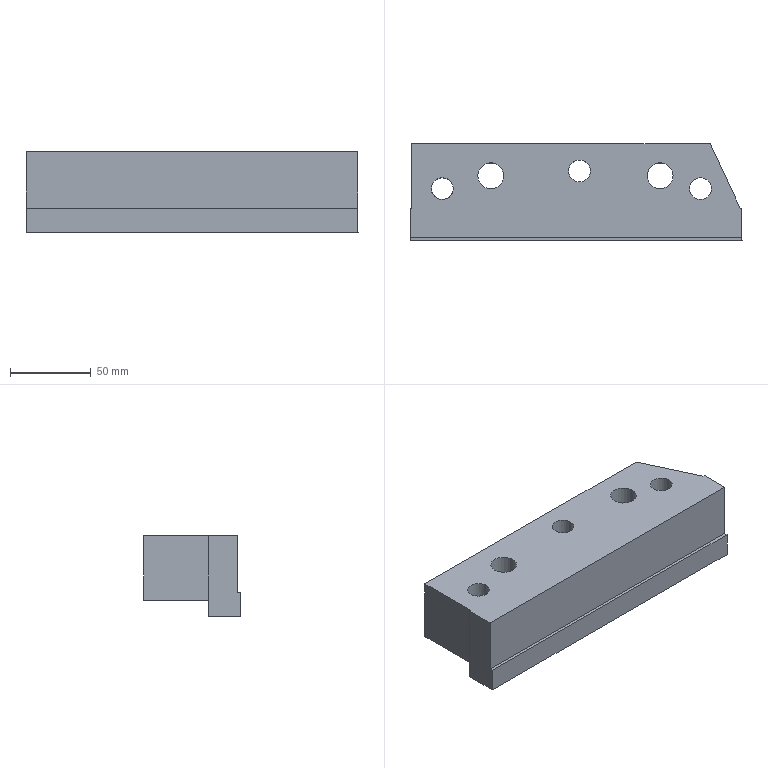Part | NX | features solid 2 | 1 solid | 23 faces | box 205.676 x 60.004 x 50 mm | volume 461052 mm3 | plane 12 | cylinder 8 | spline 3 | commonest cylinder face diameters 13.5 x3 19.5 x3 16 x2
STEP:
#1=CARTESIAN_POINT('',(205.675,-58.001,43.));
#2=VERTEX_POINT('',#1);
#3=CARTESIAN_POINT('',(205.675,-58.001,8.));
#4=VERTEX_POINT('',#3);
#5=CARTESIAN_POINT('',(205.675,-58.001,25.5));
#6=DIRECTION('',(0.,0.,-1.));
#7=VECTOR('',#6,1000.);
#8=LINE('',#5,#7);
#9=EDGE_CURVE('',#2,#4,#8,.T.);
#10=ORIENTED_EDGE('',*,*,#9,.F.);
#11=CARTESIAN_POINT('',(0.,-58.,43.));
#12=VERTEX_POINT('',#11);
#13=CARTESIAN_POINT('',(205.675,-58.001,43.));
#14=CARTESIAN_POINT('',(137.117,-58.009,43.));
#15=CARTESIAN_POINT('',(68.559,-58.,43.));
#16=CARTESIAN_POINT('',(0.,-58.,43.));
#17=B_SPLINE_CURVE_WITH_KNOTS('',3,(#13,#14,#15,#16),.UNSPECIFIED.,.F.,.F.,(4,4),(0.7842,1.),.UNSPECIFIED.);
#18=EDGE_CURVE('',#2,#12,#17,.T.);
#19=ORIENTED_EDGE('',*,*,#18,.T.);
#20=CARTESIAN_POINT('',(0.,-58.,8.));
#21=VERTEX_POINT('',#20);
#22=CARTESIAN_POINT('',(0.,-58.,25.5));
#23=DIRECTION('',(0.,0.,-1.));
#24=VECTOR('',#23,1000.);
#25=LINE('',#22,#24);
#26=EDGE_CURVE('',#12,#21,#25,.T.);
#27=ORIENTED_EDGE('',*,*,#26,.T.);
#28=CARTESIAN_POINT('',(205.675,-58.001,8.));
#29=CARTESIAN_POINT('',(137.117,-58.009,8.));
#30=CARTESIAN_POINT('',(68.559,-58.,8.));
#31=CARTESIAN_POINT('',(0.,-58.,8.));
#32=B_SPLINE_CURVE_WITH_KNOTS('',3,(#28,#29,#30,#31),.UNSPECIFIED.,.F.,.F.,(4,4),(0.7842,1.),.UNSPECIFIED.);
#33=EDGE_CURVE('',#4,#21,#32,.T.);
#34=ORIENTED_EDGE('',*,*,#33,.F.);
#35=EDGE_LOOP('',(#10,#19,#27,#34));
#36=FACE_BOUND('',#35,.T.);
#37=CARTESIAN_POINT('',(205.675,-58.001,43.));
#38=CARTESIAN_POINT('',(205.675,-58.001,8.));
#39=CARTESIAN_POINT('',(137.117,-58.009,43.));
#40=CARTESIAN_POINT('',(137.117,-58.009,8.));
#41=CARTESIAN_POINT('',(68.559,-58.,43.));
#42=CARTESIAN_POINT('',(68.559,-58.,8.));
#43=CARTESIAN_POINT('',(0.,-58.,43.));
#44=CARTESIAN_POINT('',(0.,-58.,8.));
#45=B_SPLINE_SURFACE_WITH_KNOTS('',3,1,((#37,#38),(#39,#40),(#41,#42),(#43,#44)),.SURF_OF_LINEAR_EXTRUSION.,.F.,.F.,.F.,(4,4),(2,2),(0.7842,1.),(0.,1.),.PIECEWISE_BEZIER_KNOTS.);
#46=ADVANCED_FACE('',(#36),#45,.T.);
#47=CARTESIAN_POINT('',(58.,-20.,43.));
#48=VERTEX_POINT('',#47);
#49=CARTESIAN_POINT('',(50.,-20.,43.));
#50=DIRECTION('',(0.,0.,1.));
#51=DIRECTION('',(1.,0.,0.));
#52=AXIS2_PLACEMENT_3D('',#49,#50,#51);
#53=CIRCLE('',#52,8.);
#54=EDGE_CURVE('',#48,#48,#53,.T.);
#55=ORIENTED_EDGE('',*,*,#54,.F.);
#56=EDGE_LOOP('',(#55));
#57=FACE_BOUND('',#56,.T.);
#58=CARTESIAN_POINT('',(147.,-20.,43.));
#59=VERTEX_POINT('',#58);
#60=CARTESIAN_POINT('',(155.,-20.,43.));
#61=DIRECTION('',(0.,0.,-1.));
#62=DIRECTION('',(-1.,0.,0.));
#63=AXIS2_PLACEMENT_3D('',#60,#61,#62);
#64=CIRCLE('',#63,8.);
#65=EDGE_CURVE('',#59,#59,#64,.T.);
#66=ORIENTED_EDGE('',*,*,#65,.T.);
#67=EDGE_LOOP('',(#66));
#68=FACE_BOUND('',#67,.T.);
#69=CARTESIAN_POINT('',(26.75,-28.,43.));
#70=VERTEX_POINT('',#69);
#71=CARTESIAN_POINT('',(20.,-28.,43.));
#72=DIRECTION('',(0.,0.,1.));
#73=DIRECTION('',(1.,0.,0.));
#74=AXIS2_PLACEMENT_3D('',#71,#72,#73);
#75=CIRCLE('',#74,6.75);
#76=EDGE_CURVE('',#70,#70,#75,.T.);
#77=ORIENTED_EDGE('',*,*,#76,.F.);
#78=EDGE_LOOP('',(#77));
#79=FACE_BOUND('',#78,.T.);
#80=CARTESIAN_POINT('',(98.25,-17.,43.));
#81=VERTEX_POINT('',#80);
#82=CARTESIAN_POINT('',(105.,-17.,43.));
#83=DIRECTION('',(0.,0.,-1.));
#84=DIRECTION('',(-1.,0.,0.));
#85=AXIS2_PLACEMENT_3D('',#82,#83,#84);
#86=CIRCLE('',#85,6.75);
#87=EDGE_CURVE('',#81,#81,#86,.T.);
#88=ORIENTED_EDGE('',*,*,#87,.T.);
#89=EDGE_LOOP('',(#88));
#90=FACE_BOUND('',#89,.T.);
#91=CARTESIAN_POINT('',(173.25,-28.,43.));
#92=VERTEX_POINT('',#91);
#93=CARTESIAN_POINT('',(180.,-28.,43.));
#94=DIRECTION('',(0.,0.,-1.));
#95=DIRECTION('',(-1.,0.,0.));
#96=AXIS2_PLACEMENT_3D('',#93,#94,#95);
#97=CIRCLE('',#96,6.75);
#98=EDGE_CURVE('',#92,#92,#97,.T.);
#99=ORIENTED_EDGE('',*,*,#98,.T.);
#100=EDGE_LOOP('',(#99));
#101=FACE_BOUND('',#100,.T.);
#102=CARTESIAN_POINT('',(1.,-40.,43.));
#103=VERTEX_POINT('',#102);
#104=CARTESIAN_POINT('',(1.,0.,43.));
#105=VERTEX_POINT('',#104);
#106=CARTESIAN_POINT('',(1.,-1.,43.));
#107=DIRECTION('',(0.,1.,0.));
#108=VECTOR('',#107,1000.);
#109=LINE('',#106,#108);
#110=EDGE_CURVE('',#103,#105,#109,.T.);
#111=ORIENTED_EDGE('',*,*,#110,.F.);
#112=CARTESIAN_POINT('',(0.,-40.,43.));
#113=VERTEX_POINT('',#112);
#114=CARTESIAN_POINT('',(0.,-40.,43.));
#115=CARTESIAN_POINT('',(0.3333,-40.,43.));
#116=CARTESIAN_POINT('',(0.6667,-40.,43.));
#117=CARTESIAN_POINT('',(1.,-40.,43.));
#118=B_SPLINE_CURVE_WITH_KNOTS('',3,(#114,#115,#116,#117),.UNSPECIFIED.,.F.,.F.,(4,4),(0.,0.001),.UNSPECIFIED.);
#119=EDGE_CURVE('',#103,#113,#118,.F.);
#120=ORIENTED_EDGE('',*,*,#119,.T.);
#121=CARTESIAN_POINT('',(0.,0.,43.));
#122=DIRECTION('',(0.,-1.,0.));
#123=VECTOR('',#122,1000.);
#124=LINE('',#121,#123);
#125=EDGE_CURVE('',#113,#12,#124,.T.);
#126=ORIENTED_EDGE('',*,*,#125,.T.);
#127=ORIENTED_EDGE('',*,*,#18,.F.);
#128=CARTESIAN_POINT('',(205.675,-40.001,43.));
#129=VERTEX_POINT('',#128);
#130=CARTESIAN_POINT('',(205.668,84.753,43.));
#131=DIRECTION('',(0.00005304,-1.,0.));
#132=VECTOR('',#131,1000.);
#133=LINE('',#130,#132);
#134=EDGE_CURVE('',#129,#2,#133,.T.);
#135=ORIENTED_EDGE('',*,*,#134,.F.);
#136=CARTESIAN_POINT('',(204.571,-40.001,43.));
#137=VERTEX_POINT('',#136);
#138=CARTESIAN_POINT('',(205.675,-40.001,43.));
#139=CARTESIAN_POINT('',(205.307,-40.001,43.));
#140=CARTESIAN_POINT('',(204.939,-40.001,43.));
#141=CARTESIAN_POINT('',(204.571,-40.001,43.));
#142=B_SPLINE_CURVE_WITH_KNOTS('',3,(#138,#139,#140,#141),.UNSPECIFIED.,.F.,.F.,(4,4),(0.,0.001103),.UNSPECIFIED.);
#143=EDGE_CURVE('',#129,#137,#142,.T.);
#144=ORIENTED_EDGE('',*,*,#143,.T.);
#145=CARTESIAN_POINT('',(185.918,0.,43.));
#146=VERTEX_POINT('',#145);
#147=CARTESIAN_POINT('',(186.538,-1.329,43.));
#148=DIRECTION('',(0.4226,-0.9063,0.));
#149=VECTOR('',#148,1000.);
#150=LINE('',#147,#149);
#151=EDGE_CURVE('',#137,#146,#150,.F.);
#152=ORIENTED_EDGE('',*,*,#151,.T.);
#153=CARTESIAN_POINT('',(0.,0.,43.));
#154=DIRECTION('',(1.,0.,0.));
#155=VECTOR('',#154,1000.);
#156=LINE('',#153,#155);
#157=EDGE_CURVE('',#105,#146,#156,.T.);
#158=ORIENTED_EDGE('',*,*,#157,.F.);
#159=EDGE_LOOP('',(#111,#120,#126,#127,#135,#144,#152,#158));
#160=FACE_BOUND('',#159,.T.);
#161=CARTESIAN_POINT('',(396.872,84.764,43.));
#162=DIRECTION('',(0.,0.,-1.));
#163=DIRECTION('',(1.,0.,0.));
#164=AXIS2_PLACEMENT_3D('',#161,#162,#163);
#165=PLANE('',#164);
#166=ADVANCED_FACE('',(#57,#68,#79,#90,#101,#160),#165,.F.);
#167=CARTESIAN_POINT('',(205.675,-40.001,-7.));
#168=VERTEX_POINT('',#167);
#169=CARTESIAN_POINT('',(70.,-40.002,-7.));
#170=VERTEX_POINT('',#169);
#171=CARTESIAN_POINT('',(222.421,-40.,-7.));
#172=CARTESIAN_POINT('',(215.62,-40.001,-7.));
#173=CARTESIAN_POINT('',(208.82,-40.001,-7.));
#174=CARTESIAN_POINT('',(202.019,-40.001,-7.));
#175=CARTESIAN_POINT('',(201.346,-40.001,-7.));
#176=CARTESIAN_POINT('',(200.672,-40.001,-7.));
#177=CARTESIAN_POINT('',(199.999,-40.001,-7.));
#178=CARTESIAN_POINT('',(185.832,-40.002,-7.));
#179=CARTESIAN_POINT('',(171.666,-40.003,-7.));
#180=CARTESIAN_POINT('',(143.333,-40.004,-7.));
#181=CARTESIAN_POINT('',(129.167,-40.003,-7.));
#182=CARTESIAN_POINT('',(95.834,-40.003,-7.));
#183=CARTESIAN_POINT('',(76.667,-40.002,-7.));
#184=CARTESIAN_POINT('',(38.334,-40.,-7.));
#185=CARTESIAN_POINT('',(19.167,-40.,-7.));
#186=CARTESIAN_POINT('',(0.000401,-40.,-7.));
#187=CARTESIAN_POINT('',(-0.6663,-40.,-7.));
#188=CARTESIAN_POINT('',(-1.333,-40.,-7.));
#189=CARTESIAN_POINT('',(-2.,-40.,-7.));
#190=B_SPLINE_CURVE_WITH_KNOTS('',3,(#171,#172,#173,#174,#175,#176,#177,#178,#179,#180,#181,#182,#183,#184,#185,#186,#187,#188,#189),.UNSPECIFIED.,.F.,.F.,(4,3,3,2,2,2,3,4),(-0.1121,-0.0101,0.,0.2125,0.425,0.7125,1.,1.01),.UNSPECIFIED.);
#191=EDGE_CURVE('',#168,#170,#190,.T.);
#192=ORIENTED_EDGE('',*,*,#191,.F.);
#193=CARTESIAN_POINT('',(205.676,-60.001,-7.));
#194=VERTEX_POINT('',#193);
#195=CARTESIAN_POINT('',(205.668,84.753,-7.));
#196=DIRECTION('',(0.00005304,-1.,0.));
#197=VECTOR('',#196,1000.);
#198=LINE('',#195,#197);
#199=EDGE_CURVE('',#168,#194,#198,.T.);
#200=ORIENTED_EDGE('',*,*,#199,.T.);
#201=CARTESIAN_POINT('',(70.,-60.002,-7.));
#202=VERTEX_POINT('',#201);
#203=CARTESIAN_POINT('',(704.143,549.489,-7.));
#204=CARTESIAN_POINT('',(700.294,502.993,-7.));
#205=CARTESIAN_POINT('',(696.445,456.496,-7.));
#206=CARTESIAN_POINT('',(692.595,410.,-7.));
#207=CARTESIAN_POINT('',(692.458,408.343,-7.));
#208=CARTESIAN_POINT('',(692.134,405.032,-7.));
#209=CARTESIAN_POINT('',(691.827,400.886,-7.));
#210=CARTESIAN_POINT('',(691.464,397.578,-7.));
#211=CARTESIAN_POINT('',(691.402,395.086,-7.));
#212=CARTESIAN_POINT('',(690.964,392.595,-7.));
#213=CARTESIAN_POINT('',(689.408,390.517,-7.));
#214=CARTESIAN_POINT('',(686.986,389.671,-7.));
#215=CARTESIAN_POINT('',(684.487,389.581,-7.));
#216=CARTESIAN_POINT('',(681.996,389.453,-7.));
#217=CARTESIAN_POINT('',(678.704,388.96,-7.));
#218=CARTESIAN_POINT('',(674.57,388.503,-7.));
#219=CARTESIAN_POINT('',(669.673,387.535,-7.));
#220=CARTESIAN_POINT('',(664.783,386.537,-7.));
#221=CARTESIAN_POINT('',(659.995,385.127,-7.));
#222=CARTESIAN_POINT('',(655.202,383.733,-7.));
#223=CARTESIAN_POINT('',(650.55,381.923,-7.));
#224=CARTESIAN_POINT('',(646.672,380.42,-7.));
#225=CARTESIAN_POINT('',(643.662,379.005,-7.));
#226=CARTESIAN_POINT('',(641.411,377.928,-7.));
#227=CARTESIAN_POINT('',(639.156,376.862,-7.));
#228=CARTESIAN_POINT('',(636.191,375.356,-7.));
#229=CARTESIAN_POINT('',(632.576,373.295,-7.));
#230=CARTESIAN_POINT('',(629.081,371.043,-7.));
#231=CARTESIAN_POINT('',(626.283,369.244,-7.));
#232=CARTESIAN_POINT('',(624.228,367.832,-7.));
#233=CARTESIAN_POINT('',(622.21,366.363,-7.));
#234=CARTESIAN_POINT('',(619.546,364.372,-7.));
#235=CARTESIAN_POINT('',(616.368,361.691,-7.));
#236=CARTESIAN_POINT('',(612.546,358.478,-7.));
#237=CARTESIAN_POINT('',(609.042,354.922,-7.));
#238=CARTESIAN_POINT('',(606.061,352.022,-7.));
#239=CARTESIAN_POINT('',(603.887,349.505,-7.));
#240=CARTESIAN_POINT('',(602.262,347.611,-7.));
#241=CARTESIAN_POINT('',(600.634,345.722,-7.));
#242=CARTESIAN_POINT('',(598.542,343.136,-7.));
#243=CARTESIAN_POINT('',(594.998,338.518,-7.));
#244=CARTESIAN_POINT('',(589.869,331.973,-7.));
#245=CARTESIAN_POINT('',(583.732,324.105,-7.));
#246=CARTESIAN_POINT('',(578.643,317.53,-7.));
#247=CARTESIAN_POINT('',(574.554,312.279,-7.));
#248=CARTESIAN_POINT('',(570.923,306.701,-7.));
#249=CARTESIAN_POINT('',(564.822,296.785,-7.));
#250=CARTESIAN_POINT('',(557.245,281.952,-7.));
#251=CARTESIAN_POINT('',(551.45,266.325,-7.));
#252=CARTESIAN_POINT('',(548.558,255.043,-7.));
#253=CARTESIAN_POINT('',(547.23,248.523,-7.));
#254=CARTESIAN_POINT('',(546.404,243.602,-7.));
#255=CARTESIAN_POINT('',(545.685,238.665,-7.));
#256=CARTESIAN_POINT('',(544.956,233.729,-7.));
#257=CARTESIAN_POINT('',(544.163,228.804,-7.));
#258=CARTESIAN_POINT('',(543.03,222.238,-7.));
#259=CARTESIAN_POINT('',(540.604,216.007,-7.));
#260=CARTESIAN_POINT('',(537.562,210.084,-7.));
#261=CARTESIAN_POINT('',(534.784,205.926,-7.));
#262=CARTESIAN_POINT('',(532.049,202.788,-7.));
#263=CARTESIAN_POINT('',(529.701,200.432,-7.));
#264=CARTESIAN_POINT('',(527.298,198.128,-7.));
#265=CARTESIAN_POINT('',(524.699,196.054,-7.));
#266=CARTESIAN_POINT('',(521.947,194.18,-7.));
#267=CARTESIAN_POINT('',(519.13,192.405,-7.));
#268=CARTESIAN_POINT('',(515.609,190.197,-7.));
#269=CARTESIAN_POINT('',(509.995,186.628,-7.));
#270=CARTESIAN_POINT('',(505.193,183.605,-7.));
#271=CARTESIAN_POINT('',(488.347,172.979,-7.));
#272=CARTESIAN_POINT('',(470.923,162.051,-7.));
#273=CARTESIAN_POINT('',(452.433,150.371,-7.));
#274=CARTESIAN_POINT('',(445.662,146.198,-7.));
#275=CARTESIAN_POINT('',(440.606,143.035,-7.));
#276=CARTESIAN_POINT('',(435.698,139.633,-7.));
#277=CARTESIAN_POINT('',(429.565,134.565,-7.));
#278=CARTESIAN_POINT('',(422.879,127.153,-7.));
#279=CARTESIAN_POINT('',(416.014,117.403,-7.));
#280=CARTESIAN_POINT('',(409.871,107.153,-7.));
#281=CARTESIAN_POINT('',(404.995,98.493,-7.));
#282=CARTESIAN_POINT('',(400.982,91.628,-7.));
#283=CARTESIAN_POINT('',(394.857,81.39,-7.));
#284=CARTESIAN_POINT('',(385.627,66.06,-7.));
#285=CARTESIAN_POINT('',(373.359,45.597,-7.));
#286=CARTESIAN_POINT('',(361.076,25.143,-7.));
#287=CARTESIAN_POINT('',(351.863,9.803,-7.));
#288=CARTESIAN_POINT('',(346.247,0.4191,-7.));
#289=CARTESIAN_POINT('',(344.171,-2.972,-7.));
#290=CARTESIAN_POINT('',(342.561,-5.482,-7.));
#291=CARTESIAN_POINT('',(340.921,-7.974,-7.));
#292=CARTESIAN_POINT('',(338.671,-11.253,-7.));
#293=CARTESIAN_POINT('',(335.579,-15.149,-7.));
#294=CARTESIAN_POINT('',(331.771,-19.742,-7.));
#295=CARTESIAN_POINT('',(327.68,-24.086,-7.));
#296=CARTESIAN_POINT('',(323.394,-28.235,-7.));
#297=CARTESIAN_POINT('',(318.933,-32.197,-7.));
#298=CARTESIAN_POINT('',(315.035,-35.286,-7.));
#299=CARTESIAN_POINT('',(311.798,-37.595,-7.));
#300=CARTESIAN_POINT('',(308.565,-39.911,-7.));
#301=CARTESIAN_POINT('',(304.4,-42.633,-7.));
#302=CARTESIAN_POINT('',(299.148,-45.464,-7.));
#303=CARTESIAN_POINT('',(293.89,-48.284,-7.));
#304=CARTESIAN_POINT('',(289.325,-50.258,-7.));
#305=CARTESIAN_POINT('',(285.634,-51.738,-7.));
#306=CARTESIAN_POINT('',(282.879,-52.885,-7.));
#307=CARTESIAN_POINT('',(280.041,-53.8,-7.));
#308=CARTESIAN_POINT('',(277.185,-54.663,-7.));
#309=CARTESIAN_POINT('',(274.33,-55.522,-7.));
#310=CARTESIAN_POINT('',(270.488,-56.55,-7.));
#311=CARTESIAN_POINT('',(265.653,-57.72,-7.));
#312=CARTESIAN_POINT('',(260.737,-58.464,-7.));
#313=CARTESIAN_POINT('',(256.804,-59.062,-7.));
#314=CARTESIAN_POINT('',(254.337,-59.354,-7.));
#315=CARTESIAN_POINT('',(252.356,-59.521,-7.));
#316=CARTESIAN_POINT('',(250.373,-59.675,-7.));
#317=CARTESIAN_POINT('',(247.891,-59.803,-7.));
#318=CARTESIAN_POINT('',(244.911,-59.906,-7.));
#319=CARTESIAN_POINT('',(240.936,-60.021,-7.));
#320=CARTESIAN_POINT('',(235.965,-60.032,-7.));
#321=CARTESIAN_POINT('',(231.03,-59.997,-7.));
#322=CARTESIAN_POINT('',(190.708,-60.004,-7.));
#323=CARTESIAN_POINT('',(114.042,-60.004,-7.));
#324=CARTESIAN_POINT('',(38.333,-60.,-7.));
#325=CARTESIAN_POINT('',(0.,-60.,-7.));
#326=CARTESIAN_POINT('',(-46.656,-60.,-7.));
#327=CARTESIAN_POINT('',(-93.311,-60.,-7.));
#328=CARTESIAN_POINT('',(-139.967,-60.,-7.));
#329=B_SPLINE_CURVE_WITH_KNOTS('',3,(#203,#204,#205,#206,#207,#208,#209,#210,#211,#212,#213,#214,#215,#216,#217,#218,#219,#220,#221,#222,#223,#224,#225,#226,#227,#228,#229,#230,#231,#232,#233,#234,#235,#236,#237,#238,#239,#240,#241,#242,#243,#244,#245,#246,#247,#248,#249,#250,#251,#252,#253,#254,#255,#256,#257,#258,#259,#260,#261,#262,#263,#264,#265,#266,#267,#268,#269,#270,#271,#272,#273,#274,#275,#276,#277,#278,#279,#280,#281,#282,#283,#284,#285,#286,#287,#288,#289,#290,#291,#292,#293,#294,#295,#296,#297,#298,#299,#300,#301,#302,#303,#304,#305,#306,#307,#308,#309,#310,#311,#312,#313,#314,#315,#316,#317,#318,#319,#320,#321,#322,#323,#324,#325,#326,#327,#328),.UNSPECIFIED.,.F.,.F.,(4,3,1,1,1,1,1,1,1,1,1,1,1,1,1,1,1,1,1,1,1,1,1,1,1,1,1,1,1,1,1,1,1,1,1,1,1,1,1,1,1,1,1,1,1,1,1,1,1,1,1,1,1,1,1,1,1,1,1,1,1,1,1,1,1,1,1,1,1,1,1,1,1,1,1,1,1,1,1,1,1,1,1,1,1,1,1,1,1,1,1,1,1,1,1,1,1,1,1,1,1,1,1,1,1,1,1,1,1,1,1,1,1,1,1,1,1,1,3,4),(-0.15,0.,0.005347,0.01069,0.01337,0.01604,0.01871,0.02139,0.02406,0.02673,0.02941,0.03208,0.03743,0.04278,0.04812,0.05347,0.05882,0.06416,0.06951,0.07218,0.07486,0.07753,0.0802,0.08555,0.0909,0.09357,0.09624,0.09892,0.1016,0.1069,0.1123,0.1176,0.123,0.1257,0.1283,0.131,0.1337,0.139,0.1497,0.1604,0.1711,0.1764,0.1818,0.1925,0.2139,0.2353,0.246,0.2513,0.2567,0.262,0.2673,0.2727,0.278,0.2887,0.2941,0.2994,0.3048,0.3074,0.3101,0.3155,0.3181,0.3208,0.3262,0.3315,0.3422,0.3444,0.3955,0.4083,0.4147,0.4211,0.4275,0.4339,0.4467,0.4595,0.4722,0.485,0.4914,0.4978,0.5234,0.549,0.5745,0.6001,0.6065,0.6097,0.6129,0.6161,0.6193,0.6257,0.6321,0.6385,0.6448,0.6512,0.6576,0.6608,0.664,0.6704,0.6768,0.6832,0.6896,0.6928,0.696,0.6992,0.7024,0.7056,0.7088,0.7152,0.7216,0.7247,0.7279,0.7295,0.7311,0.7343,0.7375,0.7407,0.7471,0.7535,0.7566,0.8768,1.,1.15),.UNSPECIFIED.);
#330=EDGE_CURVE('',#194,#202,#329,.T.);
#331=ORIENTED_EDGE('',*,*,#330,.T.);
#332=CARTESIAN_POINT('',(0.,-60.,-7.));
#333=VERTEX_POINT('',#332);
#334=CARTESIAN_POINT('',(0.,-60.,-7.));
#335=CARTESIAN_POINT('',(23.333,-60.,-7.));
#336=CARTESIAN_POINT('',(46.667,-60.001,-7.));
#337=CARTESIAN_POINT('',(70.,-60.002,-7.));
#338=B_SPLINE_CURVE_WITH_KNOTS('',3,(#334,#335,#336,#337),.UNSPECIFIED.,.F.,.F.,(4,4),(0.,0.07),.UNSPECIFIED.);
#339=EDGE_CURVE('',#202,#333,#338,.F.);
#340=ORIENTED_EDGE('',*,*,#339,.T.);
#341=CARTESIAN_POINT('',(0.,-40.,-7.));
#342=VERTEX_POINT('',#341);
#343=CARTESIAN_POINT('',(0.,84.764,-7.));
#344=DIRECTION('',(0.,-1.,0.));
#345=VECTOR('',#344,1000.);
#346=LINE('',#343,#345);
#347=EDGE_CURVE('',#342,#333,#346,.T.);
#348=ORIENTED_EDGE('',*,*,#347,.F.);
#349=CARTESIAN_POINT('',(70.,-40.002,-7.));
#350=CARTESIAN_POINT('',(46.667,-40.001,-7.));
#351=CARTESIAN_POINT('',(23.333,-40.,-7.));
#352=CARTESIAN_POINT('',(0.,-40.,-7.));
#353=B_SPLINE_CURVE_WITH_KNOTS('',3,(#349,#350,#351,#352),.UNSPECIFIED.,.F.,.F.,(4,4),(0.,0.07),.UNSPECIFIED.);
#354=EDGE_CURVE('',#170,#342,#353,.T.);
#355=ORIENTED_EDGE('',*,*,#354,.F.);
#356=EDGE_LOOP('',(#192,#200,#331,#340,#348,#355));
#357=FACE_BOUND('',#356,.T.);
#358=CARTESIAN_POINT('',(396.872,84.764,-7.));
#359=DIRECTION('',(0.,0.,-1.));
#360=DIRECTION('',(1.,0.,0.));
#361=AXIS2_PLACEMENT_3D('',#358,#359,#360);
#362=PLANE('',#361);
#363=ADVANCED_FACE('',(#357),#362,.T.);
#364=CARTESIAN_POINT('',(205.676,-60.001,8.));
#365=VERTEX_POINT('',#364);
#366=CARTESIAN_POINT('',(205.65,429.974,8.));
#367=DIRECTION('',(-0.00005304,1.,0.));
#368=VECTOR('',#367,1000.);
#369=LINE('',#366,#368);
#370=EDGE_CURVE('',#4,#365,#369,.F.);
#371=ORIENTED_EDGE('',*,*,#370,.F.);
#372=ORIENTED_EDGE('',*,*,#33,.T.);
#373=CARTESIAN_POINT('',(0.,-60.,8.));
#374=VERTEX_POINT('',#373);
#375=CARTESIAN_POINT('',(0.,-60.,8.));
#376=DIRECTION('',(0.,1.,0.));
#377=VECTOR('',#376,1000.);
#378=LINE('',#375,#377);
#379=EDGE_CURVE('',#374,#21,#378,.T.);
#380=ORIENTED_EDGE('',*,*,#379,.F.);
#381=CARTESIAN_POINT('',(0.,-60.,8.));
#382=CARTESIAN_POINT('',(3.422,-60.,8.));
#383=CARTESIAN_POINT('',(10.636,-60.,8.));
#384=CARTESIAN_POINT('',(20.582,-60.,8.));
#385=CARTESIAN_POINT('',(29.094,-60.,8.));
#386=CARTESIAN_POINT('',(35.757,-60.001,8.));
#387=CARTESIAN_POINT('',(41.542,-60.001,8.));
#388=CARTESIAN_POINT('',(46.308,-60.001,8.));
#389=CARTESIAN_POINT('',(49.953,-60.001,8.));
#390=CARTESIAN_POINT('',(53.048,-60.001,8.));
#391=CARTESIAN_POINT('',(55.559,-60.001,8.));
#392=CARTESIAN_POINT('',(57.142,-60.001,8.));
#393=CARTESIAN_POINT('',(58.259,-60.001,8.));
#394=CARTESIAN_POINT('',(58.898,-60.001,8.));
#395=CARTESIAN_POINT('',(59.301,-60.001,8.));
#396=CARTESIAN_POINT('',(59.619,-60.001,8.));
#397=CARTESIAN_POINT('',(60.199,-60.001,8.));
#398=CARTESIAN_POINT('',(61.086,-60.001,8.));
#399=CARTESIAN_POINT('',(62.929,-60.001,8.));
#400=CARTESIAN_POINT('',(65.463,-60.001,8.));
#401=CARTESIAN_POINT('',(69.431,-60.002,8.));
#402=CARTESIAN_POINT('',(74.17,-60.002,8.));
#403=CARTESIAN_POINT('',(81.307,-60.002,8.));
#404=CARTESIAN_POINT('',(89.381,-60.002,8.));
#405=CARTESIAN_POINT('',(97.716,-60.003,8.));
#406=CARTESIAN_POINT('',(104.697,-60.003,8.));
#407=CARTESIAN_POINT('',(110.325,-60.003,8.));
#408=CARTESIAN_POINT('',(113.887,-60.003,8.));
#409=CARTESIAN_POINT('',(116.06,-60.003,8.));
#410=CARTESIAN_POINT('',(117.351,-60.003,8.));
#411=CARTESIAN_POINT('',(118.145,-60.003,8.));
#412=CARTESIAN_POINT('',(118.611,-60.003,8.));
#413=CARTESIAN_POINT('',(118.832,-60.003,8.));
#414=CARTESIAN_POINT('',(118.966,-60.003,8.));
#415=CARTESIAN_POINT('',(119.047,-60.003,8.));
#416=CARTESIAN_POINT('',(119.093,-60.003,8.));
#417=CARTESIAN_POINT('',(119.126,-60.003,8.));
#418=CARTESIAN_POINT('',(119.127,-60.003,8.));
#419=CARTESIAN_POINT('',(119.157,-60.003,8.));
#420=CARTESIAN_POINT('',(119.123,-60.003,8.));
#421=CARTESIAN_POINT('',(119.282,-60.003,8.));
#422=CARTESIAN_POINT('',(119.483,-60.003,8.));
#423=CARTESIAN_POINT('',(119.963,-60.003,8.));
#424=CARTESIAN_POINT('',(121.002,-60.003,8.));
#425=CARTESIAN_POINT('',(122.588,-60.003,8.));
#426=CARTESIAN_POINT('',(124.475,-60.003,8.));
#427=CARTESIAN_POINT('',(126.967,-60.003,8.));
#428=CARTESIAN_POINT('',(130.04,-60.004,8.));
#429=CARTESIAN_POINT('',(133.658,-60.004,8.));
#430=CARTESIAN_POINT('',(138.389,-60.004,8.));
#431=CARTESIAN_POINT('',(144.13,-60.004,8.));
#432=CARTESIAN_POINT('',(150.744,-60.004,8.));
#433=CARTESIAN_POINT('',(157.08,-60.004,8.));
#434=CARTESIAN_POINT('',(163.142,-60.004,8.));
#435=CARTESIAN_POINT('',(168.919,-60.003,8.));
#436=CARTESIAN_POINT('',(173.527,-60.003,8.));
#437=CARTESIAN_POINT('',(176.584,-60.003,8.));
#438=CARTESIAN_POINT('',(178.036,-60.003,8.));
#439=CARTESIAN_POINT('',(178.635,-60.003,8.));
#440=CARTESIAN_POINT('',(179.198,-60.003,8.));
#441=CARTESIAN_POINT('',(180.181,-60.003,8.));
#442=CARTESIAN_POINT('',(181.581,-60.003,8.));
#443=CARTESIAN_POINT('',(183.807,-60.003,8.));
#444=CARTESIAN_POINT('',(186.568,-60.003,8.));
#445=CARTESIAN_POINT('',(189.845,-60.002,8.));
#446=CARTESIAN_POINT('',(194.165,-60.002,8.));
#447=CARTESIAN_POINT('',(199.474,-60.001,8.));
#448=CARTESIAN_POINT('',(203.625,-60.001,8.));
#449=CARTESIAN_POINT('',(205.676,-60.001,8.));
#450=B_SPLINE_CURVE_WITH_KNOTS('',3,(#381,#382,#383,#384,#385,#386,#387,#388,#389,#390,#391,#392,#393,#394,#395,#396,#397,#398,#399,#400,#401,#402,#403,#404,#405,#406,#407,#408,#409,#410,#411,#412,#413,#414,#415,#416,#417,#418,#419,#420,#421,#422,#423,#424,#425,#426,#427,#428,#429,#430,#431,#432,#433,#434,#435,#436,#437,#438,#439,#440,#441,#442,#443,#444,#445,#446,#447,#448,#449),.UNSPECIFIED.,.F.,.F.,(4,1,1,1,1,1,1,1,1,1,1,1,1,1,1,1,1,1,1,1,1,1,1,1,1,1,1,1,1,1,1,1,1,1,1,1,1,1,1,1,1,1,1,1,1,1,1,1,1,1,1,1,1,1,1,1,1,1,1,1,1,1,1,1,1,1,4),(0.,0.01348,0.02695,0.03369,0.04043,0.04717,0.05054,0.05391,0.05728,0.05896,0.06065,0.06149,0.06191,0.06233,0.06254,0.06275,0.06317,0.06402,0.0657,0.06738,0.07075,0.07412,0.08086,0.0876,0.09434,0.1011,0.1078,0.1112,0.1146,0.1179,0.1196,0.1213,0.1221,0.123,0.1238,0.1242,0.1247,0.1249,0.125,0.1251,0.1253,0.1255,0.1263,0.128,0.1297,0.1314,0.1348,0.1381,0.1415,0.1482,0.155,0.1617,0.1685,0.1752,0.1819,0.1853,0.187,0.1874,0.1878,0.1887,0.1904,0.192,0.1954,0.1988,0.2022,0.2089,0.2156),.UNSPECIFIED.);
#451=EDGE_CURVE('',#365,#374,#450,.F.);
#452=ORIENTED_EDGE('',*,*,#451,.F.);
#453=EDGE_LOOP('',(#371,#372,#380,#452));
#454=FACE_BOUND('',#453,.T.);
#455=CARTESIAN_POINT('',(694.251,430.,8.));
#456=DIRECTION('',(0.,0.,1.));
#457=DIRECTION('',(-1.,0.,0.));
#458=AXIS2_PLACEMENT_3D('',#455,#456,#457);
#459=PLANE('',#458);
#460=ADVANCED_FACE('',(#454),#459,.T.);
#461=CARTESIAN_POINT('',(205.676,-60.001,0.5));
#462=DIRECTION('',(0.,0.,-1.));
#463=VECTOR('',#462,1000.);
#464=LINE('',#461,#463);
#465=EDGE_CURVE('',#365,#194,#464,.T.);
#466=ORIENTED_EDGE('',*,*,#465,.F.);
#467=ORIENTED_EDGE('',*,*,#451,.T.);
#468=CARTESIAN_POINT('',(0.,-60.,43.));
#469=DIRECTION('',(0.,0.,-1.));
#470=VECTOR('',#469,1000.);
#471=LINE('',#468,#470);
#472=EDGE_CURVE('',#374,#333,#471,.T.);
#473=ORIENTED_EDGE('',*,*,#472,.T.);
#474=ORIENTED_EDGE('',*,*,#339,.F.);
#475=ORIENTED_EDGE('',*,*,#330,.F.);
#476=EDGE_LOOP('',(#466,#467,#473,#474,#475));
#477=FACE_BOUND('',#476,.T.);
#478=CARTESIAN_POINT('',(205.676,-60.001,8.));
#479=CARTESIAN_POINT('',(205.676,-60.001,-7.));
#480=CARTESIAN_POINT('',(137.117,-60.009,8.));
#481=CARTESIAN_POINT('',(137.117,-60.009,-7.));
#482=CARTESIAN_POINT('',(68.559,-60.,8.));
#483=CARTESIAN_POINT('',(68.559,-60.,-7.));
#484=CARTESIAN_POINT('',(0.,-60.,8.));
#485=CARTESIAN_POINT('',(0.,-60.,-7.));
#486=B_SPLINE_SURFACE_WITH_KNOTS('',3,1,((#478,#479),(#480,#481),(#482,#483),(#484,#485)),.SURF_OF_LINEAR_EXTRUSION.,.F.,.F.,.F.,(4,4),(2,2),(0.7796,1.),(0.,1.),.PIECEWISE_BEZIER_KNOTS.);
#487=ADVANCED_FACE('',(#477),#486,.T.);
#488=CARTESIAN_POINT('',(1.,0.,3.));
#489=VERTEX_POINT('',#488);
#490=CARTESIAN_POINT('',(185.918,0.,3.));
#491=VERTEX_POINT('',#490);
#492=CARTESIAN_POINT('',(0.,0.,3.));
#493=DIRECTION('',(-1.,0.,0.));
#494=VECTOR('',#493,1000.);
#495=LINE('',#492,#494);
#496=EDGE_CURVE('',#489,#491,#495,.F.);
#497=ORIENTED_EDGE('',*,*,#496,.F.);
#498=CARTESIAN_POINT('',(1.,0.,43.));
#499=DIRECTION('',(0.,0.,1.));
#500=VECTOR('',#499,1000.);
#501=LINE('',#498,#500);
#502=EDGE_CURVE('',#489,#105,#501,.T.);
#503=ORIENTED_EDGE('',*,*,#502,.T.);
#504=ORIENTED_EDGE('',*,*,#157,.T.);
#505=CARTESIAN_POINT('',(185.918,0.,43.));
#506=DIRECTION('',(0.,0.,-1.));
#507=VECTOR('',#506,1000.);
#508=LINE('',#505,#507);
#509=EDGE_CURVE('',#146,#491,#508,.T.);
#510=ORIENTED_EDGE('',*,*,#509,.T.);
#511=EDGE_LOOP('',(#497,#503,#504,#510));
#512=FACE_BOUND('',#511,.T.);
#513=CARTESIAN_POINT('',(0.,0.,43.));
#514=DIRECTION('',(0.,-1.,0.));
#515=DIRECTION('',(0.,0.,-1.));
#516=AXIS2_PLACEMENT_3D('',#513,#514,#515);
#517=PLANE('',#516);
#518=ADVANCED_FACE('',(#512),#517,.F.);
#519=CARTESIAN_POINT('',(114.75,-17.,3.));
#520=VERTEX_POINT('',#519);
#521=CARTESIAN_POINT('',(105.,-17.,3.));
#522=DIRECTION('',(0.,0.,1.));
#523=DIRECTION('',(1.,0.,0.));
#524=AXIS2_PLACEMENT_3D('',#521,#522,#523);
#525=CIRCLE('',#524,9.75);
#526=EDGE_CURVE('',#520,#520,#525,.T.);
#527=ORIENTED_EDGE('',*,*,#526,.T.);
#528=EDGE_LOOP('',(#527));
#529=FACE_BOUND('',#528,.T.);
#530=CARTESIAN_POINT('',(163.,-20.,3.));
#531=VERTEX_POINT('',#530);
#532=CARTESIAN_POINT('',(155.,-20.,3.));
#533=DIRECTION('',(0.,0.,1.));
#534=DIRECTION('',(1.,0.,0.));
#535=AXIS2_PLACEMENT_3D('',#532,#533,#534);
#536=CIRCLE('',#535,8.);
#537=EDGE_CURVE('',#531,#531,#536,.T.);
#538=ORIENTED_EDGE('',*,*,#537,.T.);
#539=EDGE_LOOP('',(#538));
#540=FACE_BOUND('',#539,.T.);
#541=CARTESIAN_POINT('',(58.,-20.,3.));
#542=VERTEX_POINT('',#541);
#543=CARTESIAN_POINT('',(50.,-20.,3.));
#544=DIRECTION('',(0.,0.,1.));
#545=DIRECTION('',(1.,0.,0.));
#546=AXIS2_PLACEMENT_3D('',#543,#544,#545);
#547=CIRCLE('',#546,8.);
#548=EDGE_CURVE('',#542,#542,#547,.T.);
#549=ORIENTED_EDGE('',*,*,#548,.T.);
#550=EDGE_LOOP('',(#549));
#551=FACE_BOUND('',#550,.T.);
#552=CARTESIAN_POINT('',(29.75,-28.,3.));
#553=VERTEX_POINT('',#552);
#554=CARTESIAN_POINT('',(20.,-28.,3.));
#555=DIRECTION('',(0.,0.,1.));
#556=DIRECTION('',(1.,0.,0.));
#557=AXIS2_PLACEMENT_3D('',#554,#555,#556);
#558=CIRCLE('',#557,9.75);
#559=EDGE_CURVE('',#553,#553,#558,.T.);
#560=ORIENTED_EDGE('',*,*,#559,.T.);
#561=EDGE_LOOP('',(#560));
#562=FACE_BOUND('',#561,.T.);
#563=CARTESIAN_POINT('',(189.75,-28.,3.));
#564=VERTEX_POINT('',#563);
#565=CARTESIAN_POINT('',(180.,-28.,3.));
#566=DIRECTION('',(0.,0.,1.));
#567=DIRECTION('',(1.,0.,0.));
#568=AXIS2_PLACEMENT_3D('',#565,#566,#567);
#569=CIRCLE('',#568,9.75);
#570=EDGE_CURVE('',#564,#564,#569,.T.);
#571=ORIENTED_EDGE('',*,*,#570,.T.);
#572=EDGE_LOOP('',(#571));
#573=FACE_BOUND('',#572,.T.);
#574=CARTESIAN_POINT('',(204.571,-40.001,3.));
#575=VERTEX_POINT('',#574);
#576=CARTESIAN_POINT('',(1.,-40.,3.));
#577=VERTEX_POINT('',#576);
#578=CARTESIAN_POINT('',(219.999,-40.,3.));
#579=CARTESIAN_POINT('',(213.332,-40.001,3.));
#580=CARTESIAN_POINT('',(206.666,-40.001,3.));
#581=CARTESIAN_POINT('',(199.999,-40.001,3.));
#582=CARTESIAN_POINT('',(185.832,-40.002,3.));
#583=CARTESIAN_POINT('',(171.666,-40.003,3.));
#584=CARTESIAN_POINT('',(143.333,-40.004,3.));
#585=CARTESIAN_POINT('',(129.167,-40.003,3.));
#586=CARTESIAN_POINT('',(95.834,-40.003,3.));
#587=CARTESIAN_POINT('',(76.667,-40.002,3.));
#588=CARTESIAN_POINT('',(38.334,-40.,3.));
#589=CARTESIAN_POINT('',(19.167,-40.,3.));
#590=CARTESIAN_POINT('',(0.000401,-40.,3.));
#591=B_SPLINE_CURVE_WITH_KNOTS('',3,(#578,#579,#580,#581,#582,#583,#584,#585,#586,#587,#588,#589,#590),.UNSPECIFIED.,.F.,.F.,(4,3,2,2,2,4),(-0.1,0.,0.2125,0.425,0.7125,1.),.UNSPECIFIED.);
#592=EDGE_CURVE('',#575,#577,#591,.T.);
#593=ORIENTED_EDGE('',*,*,#592,.T.);
#594=CARTESIAN_POINT('',(1.,-1.,3.));
#595=DIRECTION('',(0.,1.,0.));
#596=VECTOR('',#595,1000.);
#597=LINE('',#594,#596);
#598=EDGE_CURVE('',#577,#489,#597,.T.);
#599=ORIENTED_EDGE('',*,*,#598,.T.);
#600=ORIENTED_EDGE('',*,*,#496,.T.);
#601=CARTESIAN_POINT('',(186.538,-1.329,3.));
#602=DIRECTION('',(0.4226,-0.9063,0.));
#603=VECTOR('',#602,1000.);
#604=LINE('',#601,#603);
#605=EDGE_CURVE('',#575,#491,#604,.F.);
#606=ORIENTED_EDGE('',*,*,#605,.F.);
#607=EDGE_LOOP('',(#593,#599,#600,#606));
#608=FACE_BOUND('',#607,.T.);
#609=CARTESIAN_POINT('',(199.999,-40.001,3.));
#610=DIRECTION('',(0.,0.,-1.));
#611=DIRECTION('',(-1.,0.,0.));
#612=AXIS2_PLACEMENT_3D('',#609,#610,#611);
#613=PLANE('',#612);
#614=ADVANCED_FACE('',(#529,#540,#551,#562,#573,#608),#613,.T.);
#615=ORIENTED_EDGE('',*,*,#125,.F.);
#616=CARTESIAN_POINT('',(0.,-40.,0.5));
#617=DIRECTION('',(0.,0.,1.));
#618=VECTOR('',#617,1000.);
#619=LINE('',#616,#618);
#620=EDGE_CURVE('',#342,#113,#619,.T.);
#621=ORIENTED_EDGE('',*,*,#620,.F.);
#622=ORIENTED_EDGE('',*,*,#347,.T.);
#623=ORIENTED_EDGE('',*,*,#472,.F.);
#624=ORIENTED_EDGE('',*,*,#379,.T.);
#625=ORIENTED_EDGE('',*,*,#26,.F.);
#626=EDGE_LOOP('',(#615,#621,#622,#623,#624,#625));
#627=FACE_BOUND('',#626,.T.);
#628=CARTESIAN_POINT('',(0.,0.,43.));
#629=DIRECTION('',(-1.,0.,0.));
#630=DIRECTION('',(0.,1.,0.));
#631=AXIS2_PLACEMENT_3D('',#628,#629,#630);
#632=PLANE('',#631);
#633=ADVANCED_FACE('',(#627),#632,.T.);
#634=ORIENTED_EDGE('',*,*,#98,.F.);
#635=EDGE_LOOP('',(#634));
#636=FACE_BOUND('',#635,.T.);
#637=CARTESIAN_POINT('',(173.25,-28.,18.));
#638=VERTEX_POINT('',#637);
#639=CARTESIAN_POINT('',(180.,-28.,18.));
#640=DIRECTION('',(0.,0.,-1.));
#641=DIRECTION('',(-1.,0.,0.));
#642=AXIS2_PLACEMENT_3D('',#639,#640,#641);
#643=CIRCLE('',#642,6.75);
#644=EDGE_CURVE('',#638,#638,#643,.T.);
#645=ORIENTED_EDGE('',*,*,#644,.T.);
#646=EDGE_LOOP('',(#645));
#647=FACE_BOUND('',#646,.T.);
#648=CARTESIAN_POINT('',(180.,-28.,43.));
#649=DIRECTION('',(0.,0.,1.));
#650=DIRECTION('',(-1.,0.,0.));
#651=AXIS2_PLACEMENT_3D('',#648,#649,#650);
#652=CYLINDRICAL_SURFACE('',#651,6.75);
#653=ADVANCED_FACE('',(#636,#647),#652,.F.);
#654=ORIENTED_EDGE('',*,*,#644,.F.);
#655=EDGE_LOOP('',(#654));
#656=FACE_BOUND('',#655,.T.);
#657=CARTESIAN_POINT('',(170.25,-28.,18.));
#658=VERTEX_POINT('',#657);
#659=CARTESIAN_POINT('',(180.,-28.,18.));
#660=DIRECTION('',(0.,0.,-1.));
#661=DIRECTION('',(-1.,0.,0.));
#662=AXIS2_PLACEMENT_3D('',#659,#660,#661);
#663=CIRCLE('',#662,9.75);
#664=EDGE_CURVE('',#658,#658,#663,.T.);
#665=ORIENTED_EDGE('',*,*,#664,.T.);
#666=EDGE_LOOP('',(#665));
#667=FACE_BOUND('',#666,.T.);
#668=CARTESIAN_POINT('',(180.,-28.,18.));
#669=DIRECTION('',(0.,0.,1.));
#670=DIRECTION('',(-1.,0.,0.));
#671=AXIS2_PLACEMENT_3D('',#668,#669,#670);
#672=PLANE('',#671);
#673=ADVANCED_FACE('',(#656,#667),#672,.F.);
#674=ORIENTED_EDGE('',*,*,#570,.F.);
#675=EDGE_LOOP('',(#674));
#676=FACE_BOUND('',#675,.T.);
#677=ORIENTED_EDGE('',*,*,#664,.F.);
#678=EDGE_LOOP('',(#677));
#679=FACE_BOUND('',#678,.T.);
#680=CARTESIAN_POINT('',(180.,-28.,-7.));
#681=DIRECTION('',(0.,0.,1.));
#682=DIRECTION('',(-1.,0.,0.));
#683=AXIS2_PLACEMENT_3D('',#680,#681,#682);
#684=CYLINDRICAL_SURFACE('',#683,9.75);
#685=ADVANCED_FACE('',(#676,#679),#684,.F.);
#686=ORIENTED_EDGE('',*,*,#87,.F.);
#687=EDGE_LOOP('',(#686));
#688=FACE_BOUND('',#687,.T.);
#689=CARTESIAN_POINT('',(98.25,-17.,18.));
#690=VERTEX_POINT('',#689);
#691=CARTESIAN_POINT('',(105.,-17.,18.));
#692=DIRECTION('',(0.,0.,-1.));
#693=DIRECTION('',(-1.,0.,0.));
#694=AXIS2_PLACEMENT_3D('',#691,#692,#693);
#695=CIRCLE('',#694,6.75);
#696=EDGE_CURVE('',#690,#690,#695,.T.);
#697=ORIENTED_EDGE('',*,*,#696,.T.);
#698=EDGE_LOOP('',(#697));
#699=FACE_BOUND('',#698,.T.);
#700=CARTESIAN_POINT('',(105.,-17.,43.));
#701=DIRECTION('',(0.,0.,1.));
#702=DIRECTION('',(-1.,0.,0.));
#703=AXIS2_PLACEMENT_3D('',#700,#701,#702);
#704=CYLINDRICAL_SURFACE('',#703,6.75);
#705=ADVANCED_FACE('',(#688,#699),#704,.F.);
#706=ORIENTED_EDGE('',*,*,#696,.F.);
#707=EDGE_LOOP('',(#706));
#708=FACE_BOUND('',#707,.T.);
#709=CARTESIAN_POINT('',(95.25,-17.,18.));
#710=VERTEX_POINT('',#709);
#711=CARTESIAN_POINT('',(105.,-17.,18.));
#712=DIRECTION('',(0.,0.,-1.));
#713=DIRECTION('',(-1.,0.,0.));
#714=AXIS2_PLACEMENT_3D('',#711,#712,#713);
#715=CIRCLE('',#714,9.75);
#716=EDGE_CURVE('',#710,#710,#715,.T.);
#717=ORIENTED_EDGE('',*,*,#716,.T.);
#718=EDGE_LOOP('',(#717));
#719=FACE_BOUND('',#718,.T.);
#720=CARTESIAN_POINT('',(105.,-17.,18.));
#721=DIRECTION('',(0.,0.,1.));
#722=DIRECTION('',(-1.,0.,0.));
#723=AXIS2_PLACEMENT_3D('',#720,#721,#722);
#724=PLANE('',#723);
#725=ADVANCED_FACE('',(#708,#719),#724,.F.);
#726=ORIENTED_EDGE('',*,*,#526,.F.);
#727=EDGE_LOOP('',(#726));
#728=FACE_BOUND('',#727,.T.);
#729=ORIENTED_EDGE('',*,*,#716,.F.);
#730=EDGE_LOOP('',(#729));
#731=FACE_BOUND('',#730,.T.);
#732=CARTESIAN_POINT('',(105.,-17.,-7.));
#733=DIRECTION('',(0.,0.,1.));
#734=DIRECTION('',(-1.,0.,0.));
#735=AXIS2_PLACEMENT_3D('',#732,#733,#734);
#736=CYLINDRICAL_SURFACE('',#735,9.75);
#737=ADVANCED_FACE('',(#728,#731),#736,.F.);
#738=CARTESIAN_POINT('',(20.,-34.75,23.));
#739=VERTEX_POINT('',#738);
#740=CARTESIAN_POINT('',(20.,-28.,23.));
#741=DIRECTION('',(0.,0.,-1.));
#742=DIRECTION('',(0.,-1.,0.));
#743=AXIS2_PLACEMENT_3D('',#740,#741,#742);
#744=CIRCLE('',#743,6.75);
#745=EDGE_CURVE('',#739,#739,#744,.T.);
#746=ORIENTED_EDGE('',*,*,#745,.T.);
#747=EDGE_LOOP('',(#746));
#748=FACE_BOUND('',#747,.T.);
#749=ORIENTED_EDGE('',*,*,#76,.T.);
#750=EDGE_LOOP('',(#749));
#751=FACE_BOUND('',#750,.T.);
#752=CARTESIAN_POINT('',(20.,-28.,48.));
#753=DIRECTION('',(0.,0.,1.));
#754=DIRECTION('',(0.,-1.,0.));
#755=AXIS2_PLACEMENT_3D('',#752,#753,#754);
#756=CYLINDRICAL_SURFACE('',#755,6.75);
#757=ADVANCED_FACE('',(#748,#751),#756,.F.);
#758=ORIENTED_EDGE('',*,*,#745,.F.);
#759=EDGE_LOOP('',(#758));
#760=FACE_BOUND('',#759,.T.);
#761=CARTESIAN_POINT('',(20.,-37.75,23.));
#762=VERTEX_POINT('',#761);
#763=CARTESIAN_POINT('',(20.,-28.,23.));
#764=DIRECTION('',(0.,0.,-1.));
#765=DIRECTION('',(0.,-1.,0.));
#766=AXIS2_PLACEMENT_3D('',#763,#764,#765);
#767=CIRCLE('',#766,9.75);
#768=EDGE_CURVE('',#762,#762,#767,.T.);
#769=ORIENTED_EDGE('',*,*,#768,.T.);
#770=EDGE_LOOP('',(#769));
#771=FACE_BOUND('',#770,.T.);
#772=CARTESIAN_POINT('',(20.,-28.,23.));
#773=DIRECTION('',(0.,0.,1.));
#774=DIRECTION('',(0.,-1.,0.));
#775=AXIS2_PLACEMENT_3D('',#772,#773,#774);
#776=PLANE('',#775);
#777=ADVANCED_FACE('',(#760,#771),#776,.F.);
#778=ORIENTED_EDGE('',*,*,#559,.F.);
#779=EDGE_LOOP('',(#778));
#780=FACE_BOUND('',#779,.T.);
#781=ORIENTED_EDGE('',*,*,#768,.F.);
#782=EDGE_LOOP('',(#781));
#783=FACE_BOUND('',#782,.T.);
#784=CARTESIAN_POINT('',(20.,-28.,-2.));
#785=DIRECTION('',(0.,0.,1.));
#786=DIRECTION('',(0.,-1.,0.));
#787=AXIS2_PLACEMENT_3D('',#784,#785,#786);
#788=CYLINDRICAL_SURFACE('',#787,9.75);
#789=ADVANCED_FACE('',(#780,#783),#788,.F.);
#790=ORIENTED_EDGE('',*,*,#537,.F.);
#791=EDGE_LOOP('',(#790));
#792=FACE_BOUND('',#791,.T.);
#793=ORIENTED_EDGE('',*,*,#65,.F.);
#794=EDGE_LOOP('',(#793));
#795=FACE_BOUND('',#794,.T.);
#796=CARTESIAN_POINT('',(155.,-20.,-7.));
#797=DIRECTION('',(0.,0.,1.));
#798=DIRECTION('',(-1.,0.,0.));
#799=AXIS2_PLACEMENT_3D('',#796,#797,#798);
#800=CYLINDRICAL_SURFACE('',#799,8.);
#801=ADVANCED_FACE('',(#792,#795),#800,.F.);
#802=ORIENTED_EDGE('',*,*,#548,.F.);
#803=EDGE_LOOP('',(#802));
#804=FACE_BOUND('',#803,.T.);
#805=ORIENTED_EDGE('',*,*,#54,.T.);
#806=EDGE_LOOP('',(#805));
#807=FACE_BOUND('',#806,.T.);
#808=CARTESIAN_POINT('',(50.,-20.,-2.));
#809=DIRECTION('',(0.,0.,1.));
#810=DIRECTION('',(0.,-1.,0.));
#811=AXIS2_PLACEMENT_3D('',#808,#809,#810);
#812=CYLINDRICAL_SURFACE('',#811,8.);
#813=ADVANCED_FACE('',(#804,#807),#812,.F.);
#814=ORIENTED_EDGE('',*,*,#354,.T.);
#815=ORIENTED_EDGE('',*,*,#620,.T.);
#816=ORIENTED_EDGE('',*,*,#119,.F.);
#817=CARTESIAN_POINT('',(1.,-40.,23.));
#818=DIRECTION('',(0.,0.,1.));
#819=VECTOR('',#818,1000.);
#820=LINE('',#817,#819);
#821=EDGE_CURVE('',#103,#577,#820,.F.);
#822=ORIENTED_EDGE('',*,*,#821,.T.);
#823=ORIENTED_EDGE('',*,*,#592,.F.);
#824=CARTESIAN_POINT('',(204.571,-40.001,23.));
#825=DIRECTION('',(0.,0.,1.));
#826=VECTOR('',#825,1000.);
#827=LINE('',#824,#826);
#828=EDGE_CURVE('',#575,#137,#827,.T.);
#829=ORIENTED_EDGE('',*,*,#828,.T.);
#830=ORIENTED_EDGE('',*,*,#143,.F.);
#831=CARTESIAN_POINT('',(205.675,-40.001,-2.));
#832=DIRECTION('',(0.,0.,1.));
#833=VECTOR('',#832,1000.);
#834=LINE('',#831,#833);
#835=EDGE_CURVE('',#129,#168,#834,.F.);
#836=ORIENTED_EDGE('',*,*,#835,.T.);
#837=ORIENTED_EDGE('',*,*,#191,.T.);
#838=EDGE_LOOP('',(#814,#815,#816,#822,#823,#829,#830,#836,#837));
#839=FACE_BOUND('',#838,.T.);
#840=CARTESIAN_POINT('',(205.675,-40.001,-7.));
#841=CARTESIAN_POINT('',(205.675,-40.001,43.));
#842=CARTESIAN_POINT('',(137.116,-40.005,-7.));
#843=CARTESIAN_POINT('',(137.116,-40.005,43.));
#844=CARTESIAN_POINT('',(68.558,-40.001,-7.));
#845=CARTESIAN_POINT('',(68.558,-40.001,43.));
#846=CARTESIAN_POINT('',(0.,-40.,-7.));
#847=CARTESIAN_POINT('',(0.,-40.,43.));
#848=B_SPLINE_SURFACE_WITH_KNOTS('',3,1,((#840,#841),(#842,#843),(#844,#845),(#846,#847)),.SURF_OF_LINEAR_EXTRUSION.,.F.,.F.,.F.,(4,4),(2,2),(-0.02838,1.),(0.,1.),.PIECEWISE_BEZIER_KNOTS.);
#849=ADVANCED_FACE('',(#839),#848,.T.);
#850=ORIENTED_EDGE('',*,*,#199,.F.);
#851=ORIENTED_EDGE('',*,*,#835,.F.);
#852=ORIENTED_EDGE('',*,*,#134,.T.);
#853=ORIENTED_EDGE('',*,*,#9,.T.);
#854=ORIENTED_EDGE('',*,*,#370,.T.);
#855=ORIENTED_EDGE('',*,*,#465,.T.);
#856=EDGE_LOOP('',(#850,#851,#852,#853,#854,#855));
#857=FACE_BOUND('',#856,.T.);
#858=CARTESIAN_POINT('',(205.675,-40.001,-7.));
#859=DIRECTION('',(1.,0.00005304,0.));
#860=DIRECTION('',(-0.00005304,1.,0.));
#861=AXIS2_PLACEMENT_3D('',#858,#859,#860);
#862=PLANE('',#861);
#863=ADVANCED_FACE('',(#857),#862,.T.);
#864=ORIENTED_EDGE('',*,*,#151,.F.);
#865=ORIENTED_EDGE('',*,*,#828,.F.);
#866=ORIENTED_EDGE('',*,*,#605,.T.);
#867=ORIENTED_EDGE('',*,*,#509,.F.);
#868=EDGE_LOOP('',(#864,#865,#866,#867));
#869=FACE_BOUND('',#868,.T.);
#870=CARTESIAN_POINT('',(186.538,-1.329,3.));
#871=DIRECTION('',(-0.9063,-0.4226,0.));
#872=DIRECTION('',(0.4226,-0.9063,0.));
#873=AXIS2_PLACEMENT_3D('',#870,#871,#872);
#874=PLANE('',#873);
#875=ADVANCED_FACE('',(#869),#874,.F.);
#876=ORIENTED_EDGE('',*,*,#598,.F.);
#877=ORIENTED_EDGE('',*,*,#821,.F.);
#878=ORIENTED_EDGE('',*,*,#110,.T.);
#879=ORIENTED_EDGE('',*,*,#502,.F.);
#880=EDGE_LOOP('',(#876,#877,#878,#879));
#881=FACE_BOUND('',#880,.T.);
#882=CARTESIAN_POINT('',(1.,-1.,43.));
#883=DIRECTION('',(1.,0.,0.));
#884=DIRECTION('',(0.,0.,-1.));
#885=AXIS2_PLACEMENT_3D('',#882,#883,#884);
#886=PLANE('',#885);
#887=ADVANCED_FACE('',(#881),#886,.F.);
#888=CLOSED_SHELL('',(#46,#166,#363,#460,#487,#518,#614,#633,#653,#673,#685,#705,#725,#737,#757,#777,#789,#801,#813,#849,#863,#875,#887));
#889=MANIFOLD_SOLID_BREP('',#888);
#890=(LENGTH_UNIT()NAMED_UNIT(*)SI_UNIT(.MILLI.,.METRE.));
#891=UNCERTAINTY_MEASURE_WITH_UNIT(LENGTH_MEASURE(0.0508),#890,'','');
#892=(NAMED_UNIT(*)PLANE_ANGLE_UNIT()SI_UNIT($,.RADIAN.));
#893=(NAMED_UNIT(*)SI_UNIT($,.STERADIAN.)SOLID_ANGLE_UNIT());
#894=(GEOMETRIC_REPRESENTATION_CONTEXT(3)GLOBAL_UNCERTAINTY_ASSIGNED_CONTEXT((#891))GLOBAL_UNIT_ASSIGNED_CONTEXT((#890,#892,#893))REPRESENTATION_CONTEXT('',''));
#895=ADVANCED_BREP_SHAPE_REPRESENTATION('',(#889),#894);